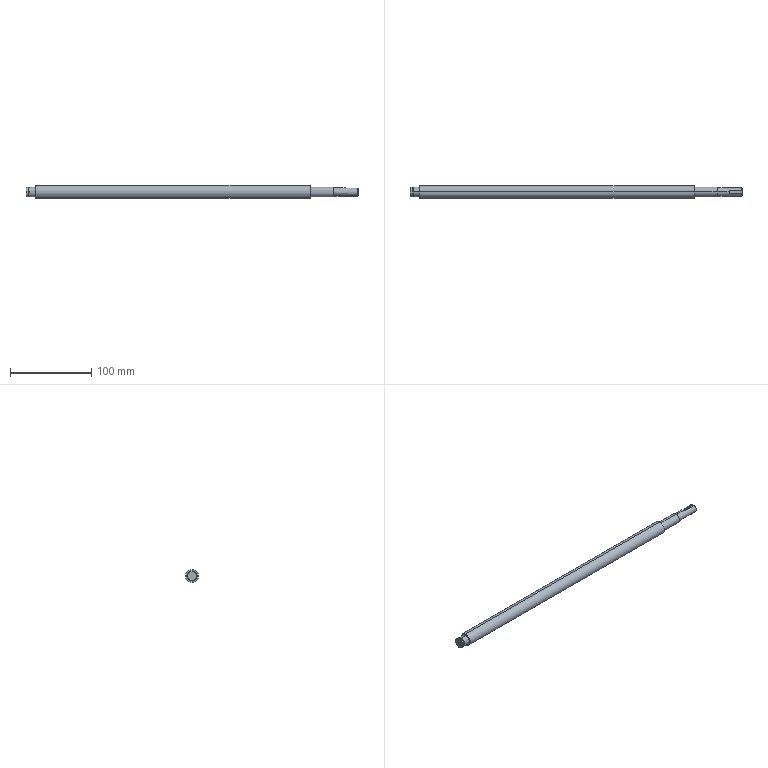Part | SolidWorks | features BaseBody 1 | 1 solid | 34 faces | box 409 x 16 x 16 mm | volume 74846 mm3 | cylinder 13 | plane 10 | torus 6 | cone 5 | commonest cylinder face diameters 12 x6 10 x2 11.5 x2 16 x2 3 x1
STEP:
#1=CARTESIAN_POINT('',(379.3,0.,-5.));
#2=VERTEX_POINT('',#1);
#3=CARTESIAN_POINT('',(379.3,0.,5.));
#4=VERTEX_POINT('',#3);
#5=CARTESIAN_POINT('',(379.3,0.,0.));
#6=DIRECTION('',(1.,0.,0.));
#7=DIRECTION('',(0.,0.,-1.));
#8=AXIS2_PLACEMENT_3D('',#5,#6,#7);
#9=CIRCLE('',#8,5.);
#10=EDGE_CURVE('',#2,#4,#9,.T.);
#11=ORIENTED_EDGE('',*,*,#10,.T.);
#12=CARTESIAN_POINT('',(393.,0.000000043,5.));
#13=VERTEX_POINT('',#12);
#14=CARTESIAN_POINT('',(409.,0.,5.));
#15=DIRECTION('',(1.,0.,0.));
#16=VECTOR('',#15,1000.);
#17=LINE('',#14,#16);
#18=EDGE_CURVE('',#4,#13,#17,.T.);
#19=ORIENTED_EDGE('',*,*,#18,.T.);
#20=CARTESIAN_POINT('',(394.5,1.5,4.77));
#21=VERTEX_POINT('',#20);
#22=CARTESIAN_POINT('',(393.,0.000000043,5.));
#23=CARTESIAN_POINT('',(393.,0.09842,5.));
#24=CARTESIAN_POINT('',(393.01,0.1983,4.997));
#25=CARTESIAN_POINT('',(393.048,0.391,4.986));
#26=CARTESIAN_POINT('',(393.077,0.4848,4.977));
#27=CARTESIAN_POINT('',(393.191,0.758,4.946));
#28=CARTESIAN_POINT('',(393.301,0.9224,4.916));
#29=CARTESIAN_POINT('',(393.509,1.13,4.871));
#30=CARTESIAN_POINT('',(393.584,1.192,4.856));
#31=CARTESIAN_POINT('',(393.746,1.3,4.828));
#32=CARTESIAN_POINT('',(393.833,1.347,4.815));
#33=CARTESIAN_POINT('',(394.104,1.46,4.783));
#34=CARTESIAN_POINT('',(394.301,1.5,4.77));
#35=CARTESIAN_POINT('',(394.5,1.5,4.77));
#36=B_SPLINE_CURVE_WITH_KNOTS('',3,(#22,#23,#24,#25,#26,#27,#28,#29,#30,#31,#32,#33,#34,#35),.UNSPECIFIED.,.F.,.F.,(4,2,2,2,2,2,4),(2.359,2.654,2.948,3.537,3.832,4.126,4.715),.UNSPECIFIED.);
#37=EDGE_CURVE('',#13,#21,#36,.T.);
#38=ORIENTED_EDGE('',*,*,#37,.T.);
#39=CARTESIAN_POINT('',(408.5,1.5,4.77));
#40=VERTEX_POINT('',#39);
#41=CARTESIAN_POINT('',(394.5,1.5,4.77));
#42=DIRECTION('',(1.,0.,0.));
#43=VECTOR('',#42,1000.);
#44=LINE('',#41,#43);
#45=EDGE_CURVE('',#21,#40,#44,.T.);
#46=ORIENTED_EDGE('',*,*,#45,.T.);
#47=CARTESIAN_POINT('',(408.5,0.,-5.));
#48=VERTEX_POINT('',#47);
#49=CARTESIAN_POINT('',(408.5,0.,0.));
#50=DIRECTION('',(1.,0.,0.));
#51=DIRECTION('',(0.,-0.3,0.9539));
#52=AXIS2_PLACEMENT_3D('',#49,#50,#51);
#53=CIRCLE('',#52,5.);
#54=EDGE_CURVE('',#48,#40,#53,.T.);
#55=ORIENTED_EDGE('',*,*,#54,.F.);
#56=CARTESIAN_POINT('',(409.,0.,-5.));
#57=DIRECTION('',(1.,0.,0.));
#58=VECTOR('',#57,1000.);
#59=LINE('',#56,#58);
#60=EDGE_CURVE('',#2,#48,#59,.T.);
#61=ORIENTED_EDGE('',*,*,#60,.F.);
#62=EDGE_LOOP('',(#11,#19,#38,#46,#55,#61));
#63=FACE_OUTER_BOUND('',#62,.T.);
#64=CARTESIAN_POINT('',(409.,0.,0.));
#65=DIRECTION('',(1.,0.,0.));
#66=DIRECTION('',(0.,0.,-1.));
#67=AXIS2_PLACEMENT_3D('',#64,#65,#66);
#68=CYLINDRICAL_SURFACE('',#67,5.);
#69=ADVANCED_FACE('',(#63),#68,.T.);
#70=CARTESIAN_POINT('',(0.,0.,-5.5));
#71=VERTEX_POINT('',#70);
#72=CARTESIAN_POINT('',(0.,0.,5.5));
#73=VERTEX_POINT('',#72);
#74=CARTESIAN_POINT('',(0.,0.,0.));
#75=DIRECTION('',(1.,0.,0.));
#76=DIRECTION('',(0.,0.,-1.));
#77=AXIS2_PLACEMENT_3D('',#74,#75,#76);
#78=CIRCLE('',#77,5.5);
#79=EDGE_CURVE('',#71,#73,#78,.T.);
#80=ORIENTED_EDGE('',*,*,#79,.T.);
#81=CARTESIAN_POINT('',(0.5,0.,6.));
#82=VERTEX_POINT('',#81);
#83=CARTESIAN_POINT('',(0.,0.,5.5));
#84=DIRECTION('',(0.7071,0.,0.7071));
#85=VECTOR('',#84,1000.);
#86=LINE('',#83,#85);
#87=EDGE_CURVE('',#73,#82,#86,.T.);
#88=ORIENTED_EDGE('',*,*,#87,.T.);
#89=CARTESIAN_POINT('',(0.5,0.,-6.));
#90=VERTEX_POINT('',#89);
#91=CARTESIAN_POINT('',(0.5,0.,0.));
#92=DIRECTION('',(1.,0.,0.));
#93=DIRECTION('',(0.,0.,-1.));
#94=AXIS2_PLACEMENT_3D('',#91,#92,#93);
#95=CIRCLE('',#94,6.);
#96=EDGE_CURVE('',#90,#82,#95,.T.);
#97=ORIENTED_EDGE('',*,*,#96,.F.);
#98=CARTESIAN_POINT('',(0.,0.,-5.5));
#99=DIRECTION('',(0.7071,0.,-0.7071));
#100=VECTOR('',#99,1000.);
#101=LINE('',#98,#100);
#102=EDGE_CURVE('',#71,#90,#101,.T.);
#103=ORIENTED_EDGE('',*,*,#102,.F.);
#104=EDGE_LOOP('',(#80,#88,#97,#103));
#105=FACE_OUTER_BOUND('',#104,.T.);
#106=CARTESIAN_POINT('',(0.,0.,0.));
#107=DIRECTION('',(1.,0.,0.));
#108=DIRECTION('',(0.,0.,-1.));
#109=AXIS2_PLACEMENT_3D('',#106,#107,#108);
#110=CONICAL_SURFACE('',#109,5.5,0.7854);
#111=ADVANCED_FACE('',(#105),#110,.T.);
#112=CARTESIAN_POINT('',(379.3,0.,0.));
#113=DIRECTION('',(1.,0.,0.));
#114=DIRECTION('',(0.,0.,-1.));
#115=AXIS2_PLACEMENT_3D('',#112,#113,#114);
#116=CIRCLE('',#115,5.);
#117=EDGE_CURVE('',#4,#2,#116,.T.);
#118=ORIENTED_EDGE('',*,*,#117,.F.);
#119=CARTESIAN_POINT('',(379.,0.,5.3));
#120=VERTEX_POINT('',#119);
#121=CARTESIAN_POINT('',(379.3,0.,5.3));
#122=DIRECTION('',(0.,1.,0.));
#123=DIRECTION('',(0.,0.,1.));
#124=AXIS2_PLACEMENT_3D('',#121,#122,#123);
#125=CIRCLE('',#124,0.3);
#126=EDGE_CURVE('',#4,#120,#125,.T.);
#127=ORIENTED_EDGE('',*,*,#126,.T.);
#128=CARTESIAN_POINT('',(379.,0.,-5.3));
#129=VERTEX_POINT('',#128);
#130=CARTESIAN_POINT('',(379.,0.,0.));
#131=DIRECTION('',(1.,0.,0.));
#132=DIRECTION('',(0.,0.,-1.));
#133=AXIS2_PLACEMENT_3D('',#130,#131,#132);
#134=CIRCLE('',#133,5.3);
#135=EDGE_CURVE('',#120,#129,#134,.T.);
#136=ORIENTED_EDGE('',*,*,#135,.T.);
#137=CARTESIAN_POINT('',(379.3,0.,-5.3));
#138=DIRECTION('',(0.,-1.,0.));
#139=DIRECTION('',(0.,0.,-1.));
#140=AXIS2_PLACEMENT_3D('',#137,#138,#139);
#141=CIRCLE('',#140,0.3);
#142=EDGE_CURVE('',#2,#129,#141,.T.);
#143=ORIENTED_EDGE('',*,*,#142,.F.);
#144=EDGE_LOOP('',(#118,#127,#136,#143));
#145=FACE_OUTER_BOUND('',#144,.T.);
#146=CARTESIAN_POINT('',(379.3,0.,0.));
#147=DIRECTION('',(1.,0.,0.));
#148=DIRECTION('',(0.,0.,-1.));
#149=AXIS2_PLACEMENT_3D('',#146,#147,#148);
#150=TOROIDAL_SURFACE('',#149,5.3,0.3);
#151=ADVANCED_FACE('',(#145),#150,.F.);
#152=ORIENTED_EDGE('',*,*,#96,.T.);
#153=CARTESIAN_POINT('',(2.71,0.,6.));
#154=VERTEX_POINT('',#153);
#155=CARTESIAN_POINT('',(12.,0.,6.));
#156=DIRECTION('',(1.,0.,0.));
#157=VECTOR('',#156,1000.);
#158=LINE('',#155,#157);
#159=EDGE_CURVE('',#82,#154,#158,.T.);
#160=ORIENTED_EDGE('',*,*,#159,.T.);
#161=CARTESIAN_POINT('',(2.71,0.,-6.));
#162=VERTEX_POINT('',#161);
#163=CARTESIAN_POINT('',(2.71,0.,0.));
#164=DIRECTION('',(-1.,0.,0.));
#165=DIRECTION('',(0.,0.,1.));
#166=AXIS2_PLACEMENT_3D('',#163,#164,#165);
#167=CIRCLE('',#166,6.);
#168=EDGE_CURVE('',#154,#162,#167,.T.);
#169=ORIENTED_EDGE('',*,*,#168,.T.);
#170=CARTESIAN_POINT('',(12.,0.,-6.));
#171=DIRECTION('',(1.,0.,0.));
#172=VECTOR('',#171,1000.);
#173=LINE('',#170,#172);
#174=EDGE_CURVE('',#90,#162,#173,.T.);
#175=ORIENTED_EDGE('',*,*,#174,.F.);
#176=EDGE_LOOP('',(#152,#160,#169,#175));
#177=FACE_OUTER_BOUND('',#176,.T.);
#178=CARTESIAN_POINT('',(12.,0.,0.));
#179=DIRECTION('',(1.,0.,0.));
#180=DIRECTION('',(0.,0.,-1.));
#181=AXIS2_PLACEMENT_3D('',#178,#179,#180);
#182=CYLINDRICAL_SURFACE('',#181,6.);
#183=ADVANCED_FACE('',(#177),#182,.T.);
#184=CARTESIAN_POINT('',(379.,0.,-5.387));
#185=VERTEX_POINT('',#184);
#186=CARTESIAN_POINT('',(379.,0.,5.387));
#187=VERTEX_POINT('',#186);
#188=CARTESIAN_POINT('',(379.,0.,0.));
#189=DIRECTION('',(1.,0.,0.));
#190=DIRECTION('',(0.,0.,-1.));
#191=AXIS2_PLACEMENT_3D('',#188,#189,#190);
#192=CIRCLE('',#191,5.387);
#193=EDGE_CURVE('',#185,#187,#192,.T.);
#194=ORIENTED_EDGE('',*,*,#193,.F.);
#195=CARTESIAN_POINT('',(378.387,0.,-6.));
#196=VERTEX_POINT('',#195);
#197=CARTESIAN_POINT('',(378.387,0.,-6.));
#198=DIRECTION('',(-0.7071,0.,-0.7071));
#199=VECTOR('',#198,1000.);
#200=LINE('',#197,#199);
#201=EDGE_CURVE('',#185,#196,#200,.T.);
#202=ORIENTED_EDGE('',*,*,#201,.T.);
#203=CARTESIAN_POINT('',(378.387,0.,6.));
#204=VERTEX_POINT('',#203);
#205=CARTESIAN_POINT('',(378.387,0.,0.));
#206=DIRECTION('',(1.,0.,0.));
#207=DIRECTION('',(0.,0.,-1.));
#208=AXIS2_PLACEMENT_3D('',#205,#206,#207);
#209=CIRCLE('',#208,6.);
#210=EDGE_CURVE('',#196,#204,#209,.T.);
#211=ORIENTED_EDGE('',*,*,#210,.T.);
#212=CARTESIAN_POINT('',(378.387,0.,6.));
#213=DIRECTION('',(-0.7071,0.,0.7071));
#214=VECTOR('',#213,1000.);
#215=LINE('',#212,#214);
#216=EDGE_CURVE('',#187,#204,#215,.T.);
#217=ORIENTED_EDGE('',*,*,#216,.F.);
#218=EDGE_LOOP('',(#194,#202,#211,#217));
#219=FACE_OUTER_BOUND('',#218,.T.);
#220=CARTESIAN_POINT('',(378.387,0.,0.));
#221=DIRECTION('',(-1.,0.,0.));
#222=DIRECTION('',(0.,0.,1.));
#223=AXIS2_PLACEMENT_3D('',#220,#221,#222);
#224=CONICAL_SURFACE('',#223,6.,0.7854);
#225=ADVANCED_FACE('',(#219),#224,.T.);
#226=CARTESIAN_POINT('',(2.71,0.,-5.75));
#227=VERTEX_POINT('',#226);
#228=CARTESIAN_POINT('',(2.71,0.,5.75));
#229=VERTEX_POINT('',#228);
#230=CARTESIAN_POINT('',(2.71,0.,0.));
#231=DIRECTION('',(1.,0.,0.));
#232=DIRECTION('',(0.,0.,-1.));
#233=AXIS2_PLACEMENT_3D('',#230,#231,#232);
#234=CIRCLE('',#233,5.75);
#235=EDGE_CURVE('',#227,#229,#234,.T.);
#236=ORIENTED_EDGE('',*,*,#235,.T.);
#237=CARTESIAN_POINT('',(4.,0.,5.75));
#238=VERTEX_POINT('',#237);
#239=CARTESIAN_POINT('',(409.,0.,5.75));
#240=DIRECTION('',(1.,0.,0.));
#241=VECTOR('',#240,1000.);
#242=LINE('',#239,#241);
#243=EDGE_CURVE('',#229,#238,#242,.T.);
#244=ORIENTED_EDGE('',*,*,#243,.T.);
#245=CARTESIAN_POINT('',(4.,0.,-5.75));
#246=VERTEX_POINT('',#245);
#247=CARTESIAN_POINT('',(4.,0.,0.));
#248=DIRECTION('',(1.,0.,0.));
#249=DIRECTION('',(0.,0.,-1.));
#250=AXIS2_PLACEMENT_3D('',#247,#248,#249);
#251=CIRCLE('',#250,5.75);
#252=EDGE_CURVE('',#246,#238,#251,.T.);
#253=ORIENTED_EDGE('',*,*,#252,.F.);
#254=CARTESIAN_POINT('',(409.,0.,-5.75));
#255=DIRECTION('',(1.,0.,0.));
#256=VECTOR('',#255,1000.);
#257=LINE('',#254,#256);
#258=EDGE_CURVE('',#227,#246,#257,.T.);
#259=ORIENTED_EDGE('',*,*,#258,.F.);
#260=EDGE_LOOP('',(#236,#244,#253,#259));
#261=FACE_OUTER_BOUND('',#260,.T.);
#262=CARTESIAN_POINT('',(409.,0.,0.));
#263=DIRECTION('',(1.,0.,0.));
#264=DIRECTION('',(0.,0.,-1.));
#265=AXIS2_PLACEMENT_3D('',#262,#263,#264);
#266=CYLINDRICAL_SURFACE('',#265,5.75);
#267=ADVANCED_FACE('',(#261),#266,.T.);
#268=CARTESIAN_POINT('',(350.3,0.,-6.));
#269=VERTEX_POINT('',#268);
#270=CARTESIAN_POINT('',(350.3,0.,6.));
#271=VERTEX_POINT('',#270);
#272=CARTESIAN_POINT('',(350.3,0.,0.));
#273=DIRECTION('',(1.,0.,0.));
#274=DIRECTION('',(0.,0.,-1.));
#275=AXIS2_PLACEMENT_3D('',#272,#273,#274);
#276=CIRCLE('',#275,6.);
#277=EDGE_CURVE('',#269,#271,#276,.T.);
#278=ORIENTED_EDGE('',*,*,#277,.T.);
#279=CARTESIAN_POINT('',(409.,0.,6.));
#280=DIRECTION('',(1.,0.,0.));
#281=VECTOR('',#280,1000.);
#282=LINE('',#279,#281);
#283=EDGE_CURVE('',#271,#204,#282,.T.);
#284=ORIENTED_EDGE('',*,*,#283,.T.);
#285=ORIENTED_EDGE('',*,*,#210,.F.);
#286=CARTESIAN_POINT('',(409.,0.,-6.));
#287=DIRECTION('',(1.,0.,0.));
#288=VECTOR('',#287,1000.);
#289=LINE('',#286,#288);
#290=EDGE_CURVE('',#269,#196,#289,.T.);
#291=ORIENTED_EDGE('',*,*,#290,.F.);
#292=EDGE_LOOP('',(#278,#284,#285,#291));
#293=FACE_OUTER_BOUND('',#292,.T.);
#294=CARTESIAN_POINT('',(409.,0.,0.));
#295=DIRECTION('',(1.,0.,0.));
#296=DIRECTION('',(0.,0.,-1.));
#297=AXIS2_PLACEMENT_3D('',#294,#295,#296);
#298=CYLINDRICAL_SURFACE('',#297,6.);
#299=ADVANCED_FACE('',(#293),#298,.T.);
#300=CARTESIAN_POINT('',(350.3,0.,0.));
#301=DIRECTION('',(1.,0.,0.));
#302=DIRECTION('',(0.,0.,-1.));
#303=AXIS2_PLACEMENT_3D('',#300,#301,#302);
#304=CIRCLE('',#303,6.);
#305=EDGE_CURVE('',#271,#269,#304,.T.);
#306=ORIENTED_EDGE('',*,*,#305,.F.);
#307=CARTESIAN_POINT('',(350.,0.,6.3));
#308=VERTEX_POINT('',#307);
#309=CARTESIAN_POINT('',(350.3,0.,6.3));
#310=DIRECTION('',(0.,1.,0.));
#311=DIRECTION('',(0.,0.,1.));
#312=AXIS2_PLACEMENT_3D('',#309,#310,#311);
#313=CIRCLE('',#312,0.3);
#314=EDGE_CURVE('',#271,#308,#313,.T.);
#315=ORIENTED_EDGE('',*,*,#314,.T.);
#316=CARTESIAN_POINT('',(350.,0.,-6.3));
#317=VERTEX_POINT('',#316);
#318=CARTESIAN_POINT('',(350.,0.,0.));
#319=DIRECTION('',(1.,0.,0.));
#320=DIRECTION('',(0.,0.,-1.));
#321=AXIS2_PLACEMENT_3D('',#318,#319,#320);
#322=CIRCLE('',#321,6.3);
#323=EDGE_CURVE('',#308,#317,#322,.T.);
#324=ORIENTED_EDGE('',*,*,#323,.T.);
#325=CARTESIAN_POINT('',(350.3,0.,-6.3));
#326=DIRECTION('',(0.,-1.,0.));
#327=DIRECTION('',(0.,0.,-1.));
#328=AXIS2_PLACEMENT_3D('',#325,#326,#327);
#329=CIRCLE('',#328,0.3);
#330=EDGE_CURVE('',#269,#317,#329,.T.);
#331=ORIENTED_EDGE('',*,*,#330,.F.);
#332=EDGE_LOOP('',(#306,#315,#324,#331));
#333=FACE_OUTER_BOUND('',#332,.T.);
#334=CARTESIAN_POINT('',(350.3,0.,0.));
#335=DIRECTION('',(1.,0.,0.));
#336=DIRECTION('',(0.,0.,-1.));
#337=AXIS2_PLACEMENT_3D('',#334,#335,#336);
#338=TOROIDAL_SURFACE('',#337,6.3,0.3);
#339=ADVANCED_FACE('',(#333),#338,.F.);
#340=CARTESIAN_POINT('',(4.,0.,-6.));
#341=VERTEX_POINT('',#340);
#342=CARTESIAN_POINT('',(4.,0.,6.));
#343=VERTEX_POINT('',#342);
#344=CARTESIAN_POINT('',(4.,0.,0.));
#345=DIRECTION('',(1.,0.,0.));
#346=DIRECTION('',(0.,0.,-1.));
#347=AXIS2_PLACEMENT_3D('',#344,#345,#346);
#348=CIRCLE('',#347,6.);
#349=EDGE_CURVE('',#341,#343,#348,.T.);
#350=ORIENTED_EDGE('',*,*,#349,.T.);
#351=CARTESIAN_POINT('',(11.7,0.,6.));
#352=VERTEX_POINT('',#351);
#353=CARTESIAN_POINT('',(12.,0.,6.));
#354=DIRECTION('',(1.,0.,0.));
#355=VECTOR('',#354,1000.);
#356=LINE('',#353,#355);
#357=EDGE_CURVE('',#343,#352,#356,.T.);
#358=ORIENTED_EDGE('',*,*,#357,.T.);
#359=CARTESIAN_POINT('',(11.7,0.,-6.));
#360=VERTEX_POINT('',#359);
#361=CARTESIAN_POINT('',(11.7,0.,0.));
#362=DIRECTION('',(1.,0.,0.));
#363=DIRECTION('',(0.,0.,-1.));
#364=AXIS2_PLACEMENT_3D('',#361,#362,#363);
#365=CIRCLE('',#364,6.);
#366=EDGE_CURVE('',#360,#352,#365,.T.);
#367=ORIENTED_EDGE('',*,*,#366,.F.);
#368=CARTESIAN_POINT('',(12.,0.,-6.));
#369=DIRECTION('',(1.,0.,0.));
#370=VECTOR('',#369,1000.);
#371=LINE('',#368,#370);
#372=EDGE_CURVE('',#341,#360,#371,.T.);
#373=ORIENTED_EDGE('',*,*,#372,.F.);
#374=EDGE_LOOP('',(#350,#358,#367,#373));
#375=FACE_OUTER_BOUND('',#374,.T.);
#376=CARTESIAN_POINT('',(12.,0.,0.));
#377=DIRECTION('',(1.,0.,0.));
#378=DIRECTION('',(0.,0.,-1.));
#379=AXIS2_PLACEMENT_3D('',#376,#377,#378);
#380=CYLINDRICAL_SURFACE('',#379,6.);
#381=ADVANCED_FACE('',(#375),#380,.T.);
#382=CARTESIAN_POINT('',(12.,0.,6.3));
#383=VERTEX_POINT('',#382);
#384=CARTESIAN_POINT('',(12.,0.,-6.3));
#385=VERTEX_POINT('',#384);
#386=CARTESIAN_POINT('',(12.,0.,0.));
#387=DIRECTION('',(1.,0.,0.));
#388=DIRECTION('',(0.,0.,-1.));
#389=AXIS2_PLACEMENT_3D('',#386,#387,#388);
#390=CIRCLE('',#389,6.3);
#391=EDGE_CURVE('',#383,#385,#390,.T.);
#392=ORIENTED_EDGE('',*,*,#391,.F.);
#393=CARTESIAN_POINT('',(11.7,0.,6.3));
#394=DIRECTION('',(0.,1.,0.));
#395=DIRECTION('',(0.,0.,1.));
#396=AXIS2_PLACEMENT_3D('',#393,#394,#395);
#397=CIRCLE('',#396,0.3);
#398=EDGE_CURVE('',#383,#352,#397,.T.);
#399=ORIENTED_EDGE('',*,*,#398,.T.);
#400=CARTESIAN_POINT('',(11.7,0.,0.));
#401=DIRECTION('',(1.,0.,0.));
#402=DIRECTION('',(0.,0.,-1.));
#403=AXIS2_PLACEMENT_3D('',#400,#401,#402);
#404=CIRCLE('',#403,6.);
#405=EDGE_CURVE('',#352,#360,#404,.T.);
#406=ORIENTED_EDGE('',*,*,#405,.T.);
#407=CARTESIAN_POINT('',(11.7,0.,-6.3));
#408=DIRECTION('',(0.,-1.,0.));
#409=DIRECTION('',(0.,0.,-1.));
#410=AXIS2_PLACEMENT_3D('',#407,#408,#409);
#411=CIRCLE('',#410,0.3);
#412=EDGE_CURVE('',#385,#360,#411,.T.);
#413=ORIENTED_EDGE('',*,*,#412,.F.);
#414=EDGE_LOOP('',(#392,#399,#406,#413));
#415=FACE_OUTER_BOUND('',#414,.T.);
#416=CARTESIAN_POINT('',(11.7,0.,0.));
#417=DIRECTION('',(1.,0.,0.));
#418=DIRECTION('',(0.,0.,-1.));
#419=AXIS2_PLACEMENT_3D('',#416,#417,#418);
#420=TOROIDAL_SURFACE('',#419,6.3,0.3);
#421=ADVANCED_FACE('',(#415),#420,.F.);
#422=CARTESIAN_POINT('',(12.,0.,-8.));
#423=VERTEX_POINT('',#422);
#424=CARTESIAN_POINT('',(12.,0.,8.));
#425=VERTEX_POINT('',#424);
#426=CARTESIAN_POINT('',(12.,0.,0.));
#427=DIRECTION('',(1.,0.,0.));
#428=DIRECTION('',(0.,0.,-1.));
#429=AXIS2_PLACEMENT_3D('',#426,#427,#428);
#430=CIRCLE('',#429,8.);
#431=EDGE_CURVE('',#423,#425,#430,.T.);
#432=ORIENTED_EDGE('',*,*,#431,.T.);
#433=CARTESIAN_POINT('',(350.,0.,8.));
#434=VERTEX_POINT('',#433);
#435=CARTESIAN_POINT('',(350.,0.,8.));
#436=DIRECTION('',(1.,0.,0.));
#437=VECTOR('',#436,1000.);
#438=LINE('',#435,#437);
#439=EDGE_CURVE('',#425,#434,#438,.T.);
#440=ORIENTED_EDGE('',*,*,#439,.T.);
#441=CARTESIAN_POINT('',(350.,0.,-8.));
#442=VERTEX_POINT('',#441);
#443=CARTESIAN_POINT('',(350.,0.,0.));
#444=DIRECTION('',(1.,0.,0.));
#445=DIRECTION('',(0.,0.,-1.));
#446=AXIS2_PLACEMENT_3D('',#443,#444,#445);
#447=CIRCLE('',#446,8.);
#448=EDGE_CURVE('',#442,#434,#447,.T.);
#449=ORIENTED_EDGE('',*,*,#448,.F.);
#450=CARTESIAN_POINT('',(350.,0.,-8.));
#451=DIRECTION('',(1.,0.,0.));
#452=VECTOR('',#451,1000.);
#453=LINE('',#450,#452);
#454=EDGE_CURVE('',#423,#442,#453,.T.);
#455=ORIENTED_EDGE('',*,*,#454,.F.);
#456=EDGE_LOOP('',(#432,#440,#449,#455));
#457=FACE_OUTER_BOUND('',#456,.T.);
#458=CARTESIAN_POINT('',(350.,0.,0.));
#459=DIRECTION('',(1.,0.,0.));
#460=DIRECTION('',(0.,0.,-1.));
#461=AXIS2_PLACEMENT_3D('',#458,#459,#460);
#462=CYLINDRICAL_SURFACE('',#461,8.);
#463=ADVANCED_FACE('',(#457),#462,.T.);
#464=ORIENTED_EDGE('',*,*,#431,.F.);
#465=CARTESIAN_POINT('',(12.,0.,0.));
#466=DIRECTION('',(1.,0.,0.));
#467=DIRECTION('',(0.,0.,-1.));
#468=AXIS2_PLACEMENT_3D('',#465,#466,#467);
#469=CIRCLE('',#468,8.);
#470=EDGE_CURVE('',#425,#423,#469,.T.);
#471=ORIENTED_EDGE('',*,*,#470,.F.);
#472=EDGE_LOOP('',(#464,#471));
#473=FACE_OUTER_BOUND('',#472,.T.);
#474=CARTESIAN_POINT('',(12.,0.,0.));
#475=DIRECTION('',(1.,0.,0.));
#476=DIRECTION('',(0.,0.,-1.));
#477=AXIS2_PLACEMENT_3D('',#474,#475,#476);
#478=CIRCLE('',#477,6.3);
#479=EDGE_CURVE('',#385,#383,#478,.T.);
#480=ORIENTED_EDGE('',*,*,#479,.T.);
#481=ORIENTED_EDGE('',*,*,#391,.T.);
#482=EDGE_LOOP('',(#480,#481));
#483=FACE_BOUND('',#482,.T.);
#484=CARTESIAN_POINT('',(12.,0.,0.));
#485=DIRECTION('',(1.,0.,0.));
#486=DIRECTION('',(0.,0.,-1.));
#487=AXIS2_PLACEMENT_3D('',#484,#485,#486);
#488=PLANE('',#487);
#489=ADVANCED_FACE('',(#473,#483),#488,.F.);
#490=ORIENTED_EDGE('',*,*,#439,.F.);
#491=ORIENTED_EDGE('',*,*,#470,.T.);
#492=ORIENTED_EDGE('',*,*,#454,.T.);
#493=CARTESIAN_POINT('',(350.,0.,0.));
#494=DIRECTION('',(1.,0.,0.));
#495=DIRECTION('',(0.,0.,-1.));
#496=AXIS2_PLACEMENT_3D('',#493,#494,#495);
#497=CIRCLE('',#496,8.);
#498=EDGE_CURVE('',#434,#442,#497,.T.);
#499=ORIENTED_EDGE('',*,*,#498,.F.);
#500=EDGE_LOOP('',(#490,#491,#492,#499));
#501=FACE_OUTER_BOUND('',#500,.T.);
#502=CARTESIAN_POINT('',(350.,0.,0.));
#503=DIRECTION('',(1.,0.,0.));
#504=DIRECTION('',(0.,0.,-1.));
#505=AXIS2_PLACEMENT_3D('',#502,#503,#504);
#506=CYLINDRICAL_SURFACE('',#505,8.);
#507=ADVANCED_FACE('',(#501),#506,.T.);
#508=ORIENTED_EDGE('',*,*,#398,.F.);
#509=ORIENTED_EDGE('',*,*,#479,.F.);
#510=ORIENTED_EDGE('',*,*,#412,.T.);
#511=ORIENTED_EDGE('',*,*,#366,.T.);
#512=EDGE_LOOP('',(#508,#509,#510,#511));
#513=FACE_OUTER_BOUND('',#512,.T.);
#514=CARTESIAN_POINT('',(11.7,0.,0.));
#515=DIRECTION('',(1.,0.,0.));
#516=DIRECTION('',(0.,0.,-1.));
#517=AXIS2_PLACEMENT_3D('',#514,#515,#516);
#518=TOROIDAL_SURFACE('',#517,6.3,0.3);
#519=ADVANCED_FACE('',(#513),#518,.F.);
#520=CARTESIAN_POINT('',(350.,0.,0.));
#521=DIRECTION('',(1.,0.,0.));
#522=DIRECTION('',(0.,0.,-1.));
#523=AXIS2_PLACEMENT_3D('',#520,#521,#522);
#524=CIRCLE('',#523,6.3);
#525=EDGE_CURVE('',#317,#308,#524,.T.);
#526=ORIENTED_EDGE('',*,*,#525,.F.);
#527=ORIENTED_EDGE('',*,*,#323,.F.);
#528=EDGE_LOOP('',(#526,#527));
#529=FACE_BOUND('',#528,.T.);
#530=ORIENTED_EDGE('',*,*,#448,.T.);
#531=ORIENTED_EDGE('',*,*,#498,.T.);
#532=EDGE_LOOP('',(#530,#531));
#533=FACE_OUTER_BOUND('',#532,.T.);
#534=CARTESIAN_POINT('',(350.,8.,0.));
#535=DIRECTION('',(-1.,0.,0.));
#536=DIRECTION('',(0.,0.,1.));
#537=AXIS2_PLACEMENT_3D('',#534,#535,#536);
#538=PLANE('',#537);
#539=ADVANCED_FACE('',(#529,#533),#538,.F.);
#540=ORIENTED_EDGE('',*,*,#357,.F.);
#541=CARTESIAN_POINT('',(4.,0.,0.));
#542=DIRECTION('',(1.,0.,0.));
#543=DIRECTION('',(0.,0.,-1.));
#544=AXIS2_PLACEMENT_3D('',#541,#542,#543);
#545=CIRCLE('',#544,6.);
#546=EDGE_CURVE('',#343,#341,#545,.T.);
#547=ORIENTED_EDGE('',*,*,#546,.T.);
#548=ORIENTED_EDGE('',*,*,#372,.T.);
#549=ORIENTED_EDGE('',*,*,#405,.F.);
#550=EDGE_LOOP('',(#540,#547,#548,#549));
#551=FACE_OUTER_BOUND('',#550,.T.);
#552=CARTESIAN_POINT('',(12.,0.,0.));
#553=DIRECTION('',(1.,0.,0.));
#554=DIRECTION('',(0.,0.,-1.));
#555=AXIS2_PLACEMENT_3D('',#552,#553,#554);
#556=CYLINDRICAL_SURFACE('',#555,6.);
#557=ADVANCED_FACE('',(#551),#556,.T.);
#558=ORIENTED_EDGE('',*,*,#314,.F.);
#559=ORIENTED_EDGE('',*,*,#277,.F.);
#560=ORIENTED_EDGE('',*,*,#330,.T.);
#561=ORIENTED_EDGE('',*,*,#525,.T.);
#562=EDGE_LOOP('',(#558,#559,#560,#561));
#563=FACE_OUTER_BOUND('',#562,.T.);
#564=CARTESIAN_POINT('',(350.3,0.,0.));
#565=DIRECTION('',(1.,0.,0.));
#566=DIRECTION('',(0.,0.,-1.));
#567=AXIS2_PLACEMENT_3D('',#564,#565,#566);
#568=TOROIDAL_SURFACE('',#567,6.3,0.3);
#569=ADVANCED_FACE('',(#563),#568,.F.);
#570=ORIENTED_EDGE('',*,*,#349,.F.);
#571=ORIENTED_EDGE('',*,*,#546,.F.);
#572=EDGE_LOOP('',(#570,#571));
#573=FACE_OUTER_BOUND('',#572,.T.);
#574=ORIENTED_EDGE('',*,*,#252,.T.);
#575=CARTESIAN_POINT('',(4.,0.,0.));
#576=DIRECTION('',(1.,0.,0.));
#577=DIRECTION('',(0.,0.,-1.));
#578=AXIS2_PLACEMENT_3D('',#575,#576,#577);
#579=CIRCLE('',#578,5.75);
#580=EDGE_CURVE('',#238,#246,#579,.T.);
#581=ORIENTED_EDGE('',*,*,#580,.T.);
#582=EDGE_LOOP('',(#574,#581));
#583=FACE_BOUND('',#582,.T.);
#584=CARTESIAN_POINT('',(4.,5.75,0.));
#585=DIRECTION('',(1.,0.,0.));
#586=DIRECTION('',(0.,0.,-1.));
#587=AXIS2_PLACEMENT_3D('',#584,#585,#586);
#588=PLANE('',#587);
#589=ADVANCED_FACE('',(#573,#583),#588,.F.);
#590=ORIENTED_EDGE('',*,*,#283,.F.);
#591=ORIENTED_EDGE('',*,*,#305,.T.);
#592=ORIENTED_EDGE('',*,*,#290,.T.);
#593=CARTESIAN_POINT('',(378.387,0.,0.));
#594=DIRECTION('',(1.,0.,0.));
#595=DIRECTION('',(0.,0.,-1.));
#596=AXIS2_PLACEMENT_3D('',#593,#594,#595);
#597=CIRCLE('',#596,6.);
#598=EDGE_CURVE('',#204,#196,#597,.T.);
#599=ORIENTED_EDGE('',*,*,#598,.F.);
#600=EDGE_LOOP('',(#590,#591,#592,#599));
#601=FACE_OUTER_BOUND('',#600,.T.);
#602=CARTESIAN_POINT('',(409.,0.,0.));
#603=DIRECTION('',(1.,0.,0.));
#604=DIRECTION('',(0.,0.,-1.));
#605=AXIS2_PLACEMENT_3D('',#602,#603,#604);
#606=CYLINDRICAL_SURFACE('',#605,6.);
#607=ADVANCED_FACE('',(#601),#606,.T.);
#608=ORIENTED_EDGE('',*,*,#243,.F.);
#609=CARTESIAN_POINT('',(2.71,0.,0.));
#610=DIRECTION('',(1.,0.,0.));
#611=DIRECTION('',(0.,0.,-1.));
#612=AXIS2_PLACEMENT_3D('',#609,#610,#611);
#613=CIRCLE('',#612,5.75);
#614=EDGE_CURVE('',#229,#227,#613,.T.);
#615=ORIENTED_EDGE('',*,*,#614,.T.);
#616=ORIENTED_EDGE('',*,*,#258,.T.);
#617=ORIENTED_EDGE('',*,*,#580,.F.);
#618=EDGE_LOOP('',(#608,#615,#616,#617));
#619=FACE_OUTER_BOUND('',#618,.T.);
#620=CARTESIAN_POINT('',(409.,0.,0.));
#621=DIRECTION('',(1.,0.,0.));
#622=DIRECTION('',(0.,0.,-1.));
#623=AXIS2_PLACEMENT_3D('',#620,#621,#622);
#624=CYLINDRICAL_SURFACE('',#623,5.75);
#625=ADVANCED_FACE('',(#619),#624,.T.);
#626=ORIENTED_EDGE('',*,*,#201,.F.);
#627=CARTESIAN_POINT('',(379.,0.,0.));
#628=DIRECTION('',(1.,0.,0.));
#629=DIRECTION('',(0.,0.,-1.));
#630=AXIS2_PLACEMENT_3D('',#627,#628,#629);
#631=CIRCLE('',#630,5.387);
#632=EDGE_CURVE('',#187,#185,#631,.T.);
#633=ORIENTED_EDGE('',*,*,#632,.F.);
#634=ORIENTED_EDGE('',*,*,#216,.T.);
#635=ORIENTED_EDGE('',*,*,#598,.T.);
#636=EDGE_LOOP('',(#626,#633,#634,#635));
#637=FACE_OUTER_BOUND('',#636,.T.);
#638=CARTESIAN_POINT('',(378.387,0.,0.));
#639=DIRECTION('',(-1.,0.,0.));
#640=DIRECTION('',(0.,0.,1.));
#641=AXIS2_PLACEMENT_3D('',#638,#639,#640);
#642=CONICAL_SURFACE('',#641,6.,0.7854);
#643=ADVANCED_FACE('',(#637),#642,.T.);
#644=ORIENTED_EDGE('',*,*,#235,.F.);
#645=ORIENTED_EDGE('',*,*,#614,.F.);
#646=EDGE_LOOP('',(#644,#645));
#647=FACE_BOUND('',#646,.T.);
#648=CARTESIAN_POINT('',(2.71,0.,0.));
#649=DIRECTION('',(-1.,0.,0.));
#650=DIRECTION('',(0.,0.,1.));
#651=AXIS2_PLACEMENT_3D('',#648,#649,#650);
#652=CIRCLE('',#651,6.);
#653=EDGE_CURVE('',#162,#154,#652,.T.);
#654=ORIENTED_EDGE('',*,*,#653,.F.);
#655=ORIENTED_EDGE('',*,*,#168,.F.);
#656=EDGE_LOOP('',(#654,#655));
#657=FACE_OUTER_BOUND('',#656,.T.);
#658=CARTESIAN_POINT('',(2.71,21.75,0.));
#659=DIRECTION('',(-1.,0.,0.));
#660=DIRECTION('',(0.,0.,1.));
#661=AXIS2_PLACEMENT_3D('',#658,#659,#660);
#662=PLANE('',#661);
#663=ADVANCED_FACE('',(#647,#657),#662,.F.);
#664=CARTESIAN_POINT('',(379.,0.,0.));
#665=DIRECTION('',(1.,0.,0.));
#666=DIRECTION('',(0.,0.,-1.));
#667=AXIS2_PLACEMENT_3D('',#664,#665,#666);
#668=CIRCLE('',#667,5.3);
#669=EDGE_CURVE('',#129,#120,#668,.T.);
#670=ORIENTED_EDGE('',*,*,#669,.F.);
#671=ORIENTED_EDGE('',*,*,#135,.F.);
#672=EDGE_LOOP('',(#670,#671));
#673=FACE_BOUND('',#672,.T.);
#674=ORIENTED_EDGE('',*,*,#632,.T.);
#675=ORIENTED_EDGE('',*,*,#193,.T.);
#676=EDGE_LOOP('',(#674,#675));
#677=FACE_OUTER_BOUND('',#676,.T.);
#678=CARTESIAN_POINT('',(379.,5.386,0.));
#679=DIRECTION('',(-1.,0.,0.));
#680=DIRECTION('',(0.,0.,1.));
#681=AXIS2_PLACEMENT_3D('',#678,#679,#680);
#682=PLANE('',#681);
#683=ADVANCED_FACE('',(#673,#677),#682,.F.);
#684=ORIENTED_EDGE('',*,*,#159,.F.);
#685=CARTESIAN_POINT('',(0.5,0.,0.));
#686=DIRECTION('',(1.,0.,0.));
#687=DIRECTION('',(0.,0.,-1.));
#688=AXIS2_PLACEMENT_3D('',#685,#686,#687);
#689=CIRCLE('',#688,6.);
#690=EDGE_CURVE('',#82,#90,#689,.T.);
#691=ORIENTED_EDGE('',*,*,#690,.T.);
#692=ORIENTED_EDGE('',*,*,#174,.T.);
#693=ORIENTED_EDGE('',*,*,#653,.T.);
#694=EDGE_LOOP('',(#684,#691,#692,#693));
#695=FACE_OUTER_BOUND('',#694,.T.);
#696=CARTESIAN_POINT('',(12.,0.,0.));
#697=DIRECTION('',(1.,0.,0.));
#698=DIRECTION('',(0.,0.,-1.));
#699=AXIS2_PLACEMENT_3D('',#696,#697,#698);
#700=CYLINDRICAL_SURFACE('',#699,6.);
#701=ADVANCED_FACE('',(#695),#700,.T.);
#702=ORIENTED_EDGE('',*,*,#126,.F.);
#703=ORIENTED_EDGE('',*,*,#10,.F.);
#704=ORIENTED_EDGE('',*,*,#142,.T.);
#705=ORIENTED_EDGE('',*,*,#669,.T.);
#706=EDGE_LOOP('',(#702,#703,#704,#705));
#707=FACE_OUTER_BOUND('',#706,.T.);
#708=CARTESIAN_POINT('',(379.3,0.,0.));
#709=DIRECTION('',(1.,0.,0.));
#710=DIRECTION('',(0.,0.,-1.));
#711=AXIS2_PLACEMENT_3D('',#708,#709,#710);
#712=TOROIDAL_SURFACE('',#711,5.3,0.3);
#713=ADVANCED_FACE('',(#707),#712,.F.);
#714=ORIENTED_EDGE('',*,*,#87,.F.);
#715=CARTESIAN_POINT('',(0.,0.,0.));
#716=DIRECTION('',(1.,0.,0.));
#717=DIRECTION('',(0.,0.,-1.));
#718=AXIS2_PLACEMENT_3D('',#715,#716,#717);
#719=CIRCLE('',#718,5.5);
#720=EDGE_CURVE('',#73,#71,#719,.T.);
#721=ORIENTED_EDGE('',*,*,#720,.T.);
#722=ORIENTED_EDGE('',*,*,#102,.T.);
#723=ORIENTED_EDGE('',*,*,#690,.F.);
#724=EDGE_LOOP('',(#714,#721,#722,#723));
#725=FACE_OUTER_BOUND('',#724,.T.);
#726=CARTESIAN_POINT('',(0.,0.,0.));
#727=DIRECTION('',(1.,0.,0.));
#728=DIRECTION('',(0.,0.,-1.));
#729=AXIS2_PLACEMENT_3D('',#726,#727,#728);
#730=CONICAL_SURFACE('',#729,5.5,0.7854);
#731=ADVANCED_FACE('',(#725),#730,.T.);
#732=ORIENTED_EDGE('',*,*,#18,.F.);
#733=ORIENTED_EDGE('',*,*,#117,.T.);
#734=ORIENTED_EDGE('',*,*,#60,.T.);
#735=CARTESIAN_POINT('',(408.5,-1.5,4.77));
#736=VERTEX_POINT('',#735);
#737=CARTESIAN_POINT('',(408.5,0.,0.));
#738=DIRECTION('',(1.,0.,0.));
#739=DIRECTION('',(0.,-0.3,0.9539));
#740=AXIS2_PLACEMENT_3D('',#737,#738,#739);
#741=CIRCLE('',#740,5.);
#742=EDGE_CURVE('',#736,#48,#741,.T.);
#743=ORIENTED_EDGE('',*,*,#742,.F.);
#744=CARTESIAN_POINT('',(394.5,-1.5,4.77));
#745=VERTEX_POINT('',#744);
#746=CARTESIAN_POINT('',(408.5,-1.5,4.77));
#747=DIRECTION('',(-1.,0.,0.));
#748=VECTOR('',#747,1000.);
#749=LINE('',#746,#748);
#750=EDGE_CURVE('',#736,#745,#749,.T.);
#751=ORIENTED_EDGE('',*,*,#750,.T.);
#752=CARTESIAN_POINT('',(394.5,-1.5,4.77));
#753=CARTESIAN_POINT('',(394.4,-1.5,4.77));
#754=CARTESIAN_POINT('',(394.302,-1.49,4.773));
#755=CARTESIAN_POINT('',(394.11,-1.452,4.785));
#756=CARTESIAN_POINT('',(394.014,-1.423,4.794));
#757=CARTESIAN_POINT('',(393.833,-1.347,4.815));
#758=CARTESIAN_POINT('',(393.747,-1.301,4.828));
#759=CARTESIAN_POINT('',(393.584,-1.192,4.856));
#760=CARTESIAN_POINT('',(393.508,-1.129,4.871));
#761=CARTESIAN_POINT('',(393.301,-0.9228,4.916));
#762=CARTESIAN_POINT('',(393.19,-0.7562,4.946));
#763=CARTESIAN_POINT('',(393.04,-0.3953,4.988));
#764=CARTESIAN_POINT('',(393.,-0.1971,5.));
#765=CARTESIAN_POINT('',(393.,0.000000043,5.));
#766=B_SPLINE_CURVE_WITH_KNOTS('',3,(#752,#753,#754,#755,#756,#757,#758,#759,#760,#761,#762,#763,#764,#765),.UNSPECIFIED.,.F.,.F.,(4,2,2,2,2,2,4),(0.,0.2949,0.5898,0.8847,1.18,1.769,2.359),.UNSPECIFIED.);
#767=EDGE_CURVE('',#745,#13,#766,.T.);
#768=ORIENTED_EDGE('',*,*,#767,.T.);
#769=EDGE_LOOP('',(#732,#733,#734,#743,#751,#768));
#770=FACE_OUTER_BOUND('',#769,.T.);
#771=CARTESIAN_POINT('',(409.,0.,0.));
#772=DIRECTION('',(1.,0.,0.));
#773=DIRECTION('',(0.,0.,-1.));
#774=AXIS2_PLACEMENT_3D('',#771,#772,#773);
#775=CYLINDRICAL_SURFACE('',#774,5.);
#776=ADVANCED_FACE('',(#770),#775,.T.);
#777=ORIENTED_EDGE('',*,*,#79,.F.);
#778=ORIENTED_EDGE('',*,*,#720,.F.);
#779=EDGE_LOOP('',(#777,#778));
#780=FACE_OUTER_BOUND('',#779,.T.);
#781=CARTESIAN_POINT('',(0.,0.,0.));
#782=DIRECTION('',(1.,0.,0.));
#783=DIRECTION('',(0.,0.,-1.));
#784=AXIS2_PLACEMENT_3D('',#781,#782,#783);
#785=PLANE('',#784);
#786=ADVANCED_FACE('',(#780),#785,.F.);
#787=CARTESIAN_POINT('',(409.,-1.5,4.243));
#788=VERTEX_POINT('',#787);
#789=CARTESIAN_POINT('',(409.,1.5,4.243));
#790=VERTEX_POINT('',#789);
#791=CARTESIAN_POINT('',(409.,0.,0.));
#792=DIRECTION('',(1.,0.,0.));
#793=DIRECTION('',(0.,-0.3333,0.9428));
#794=AXIS2_PLACEMENT_3D('',#791,#792,#793);
#795=CIRCLE('',#794,4.5);
#796=EDGE_CURVE('',#788,#790,#795,.T.);
#797=ORIENTED_EDGE('',*,*,#796,.F.);
#798=CARTESIAN_POINT('',(409.,-1.5,4.243));
#799=CARTESIAN_POINT('',(408.834,-1.5,4.419));
#800=CARTESIAN_POINT('',(408.668,-1.5,4.594));
#801=CARTESIAN_POINT('',(408.5,-1.5,4.77));
#802=B_SPLINE_CURVE_WITH_KNOTS('',3,(#798,#799,#800,#801),.UNSPECIFIED.,.F.,.F.,(4,4),(2.796,3.522),.UNSPECIFIED.);
#803=EDGE_CURVE('',#788,#736,#802,.T.);
#804=ORIENTED_EDGE('',*,*,#803,.T.);
#805=ORIENTED_EDGE('',*,*,#742,.T.);
#806=ORIENTED_EDGE('',*,*,#54,.T.);
#807=CARTESIAN_POINT('',(408.5,1.5,4.77));
#808=CARTESIAN_POINT('',(408.668,1.5,4.594));
#809=CARTESIAN_POINT('',(408.835,1.5,4.418));
#810=CARTESIAN_POINT('',(409.,1.5,4.243));
#811=B_SPLINE_CURVE_WITH_KNOTS('',3,(#807,#808,#809,#810),.UNSPECIFIED.,.F.,.F.,(4,4),(2.688,3.414),.UNSPECIFIED.);
#812=EDGE_CURVE('',#40,#790,#811,.T.);
#813=ORIENTED_EDGE('',*,*,#812,.T.);
#814=EDGE_LOOP('',(#797,#804,#805,#806,#813));
#815=FACE_OUTER_BOUND('',#814,.T.);
#816=CARTESIAN_POINT('',(408.5,0.,0.));
#817=DIRECTION('',(-1.,0.,0.));
#818=DIRECTION('',(0.,0.,1.));
#819=AXIS2_PLACEMENT_3D('',#816,#817,#818);
#820=CONICAL_SURFACE('',#819,5.,0.7854);
#821=ADVANCED_FACE('',(#815),#820,.T.);
#822=ORIENTED_EDGE('',*,*,#803,.F.);
#823=CARTESIAN_POINT('',(409.,-1.5,3.2));
#824=VERTEX_POINT('',#823);
#825=CARTESIAN_POINT('',(409.,-1.5,3.2));
#826=DIRECTION('',(0.,0.,1.));
#827=VECTOR('',#826,1000.);
#828=LINE('',#825,#827);
#829=EDGE_CURVE('',#824,#788,#828,.T.);
#830=ORIENTED_EDGE('',*,*,#829,.F.);
#831=CARTESIAN_POINT('',(394.5,-1.5,3.2));
#832=VERTEX_POINT('',#831);
#833=CARTESIAN_POINT('',(394.5,-1.5,3.2));
#834=DIRECTION('',(1.,0.,0.));
#835=VECTOR('',#834,1000.);
#836=LINE('',#833,#835);
#837=EDGE_CURVE('',#832,#824,#836,.T.);
#838=ORIENTED_EDGE('',*,*,#837,.F.);
#839=CARTESIAN_POINT('',(394.5,-1.5,3.2));
#840=DIRECTION('',(0.,0.,1.));
#841=VECTOR('',#840,1000.);
#842=LINE('',#839,#841);
#843=EDGE_CURVE('',#832,#745,#842,.T.);
#844=ORIENTED_EDGE('',*,*,#843,.T.);
#845=ORIENTED_EDGE('',*,*,#750,.F.);
#846=EDGE_LOOP('',(#822,#830,#838,#844,#845));
#847=FACE_OUTER_BOUND('',#846,.T.);
#848=CARTESIAN_POINT('',(394.5,-1.5,3.2));
#849=DIRECTION('',(0.,-1.,0.));
#850=DIRECTION('',(0.,0.,-1.));
#851=AXIS2_PLACEMENT_3D('',#848,#849,#850);
#852=PLANE('',#851);
#853=ADVANCED_FACE('',(#847),#852,.F.);
#854=ORIENTED_EDGE('',*,*,#843,.F.);
#855=CARTESIAN_POINT('',(394.5,1.5,3.2));
#856=VERTEX_POINT('',#855);
#857=CARTESIAN_POINT('',(394.5,0.,3.2));
#858=DIRECTION('',(0.,0.,1.));
#859=DIRECTION('',(0.,1.,0.));
#860=AXIS2_PLACEMENT_3D('',#857,#858,#859);
#861=CIRCLE('',#860,1.5);
#862=EDGE_CURVE('',#856,#832,#861,.T.);
#863=ORIENTED_EDGE('',*,*,#862,.F.);
#864=CARTESIAN_POINT('',(394.5,1.5,3.2));
#865=DIRECTION('',(0.,0.,1.));
#866=VECTOR('',#865,1000.);
#867=LINE('',#864,#866);
#868=EDGE_CURVE('',#856,#21,#867,.T.);
#869=ORIENTED_EDGE('',*,*,#868,.T.);
#870=ORIENTED_EDGE('',*,*,#37,.F.);
#871=ORIENTED_EDGE('',*,*,#767,.F.);
#872=EDGE_LOOP('',(#854,#863,#869,#870,#871));
#873=FACE_OUTER_BOUND('',#872,.T.);
#874=CARTESIAN_POINT('',(394.5,0.,3.2));
#875=DIRECTION('',(0.,0.,1.));
#876=DIRECTION('',(1.,0.,0.));
#877=AXIS2_PLACEMENT_3D('',#874,#875,#876);
#878=CYLINDRICAL_SURFACE('',#877,1.5);
#879=ADVANCED_FACE('',(#873),#878,.F.);
#880=ORIENTED_EDGE('',*,*,#868,.F.);
#881=CARTESIAN_POINT('',(409.,1.5,3.2));
#882=VERTEX_POINT('',#881);
#883=CARTESIAN_POINT('',(409.,1.5,3.2));
#884=DIRECTION('',(-1.,0.,0.));
#885=VECTOR('',#884,1000.);
#886=LINE('',#883,#885);
#887=EDGE_CURVE('',#882,#856,#886,.T.);
#888=ORIENTED_EDGE('',*,*,#887,.F.);
#889=CARTESIAN_POINT('',(409.,1.5,3.2));
#890=DIRECTION('',(0.,0.,1.));
#891=VECTOR('',#890,1000.);
#892=LINE('',#889,#891);
#893=EDGE_CURVE('',#882,#790,#892,.T.);
#894=ORIENTED_EDGE('',*,*,#893,.T.);
#895=ORIENTED_EDGE('',*,*,#812,.F.);
#896=ORIENTED_EDGE('',*,*,#45,.F.);
#897=EDGE_LOOP('',(#880,#888,#894,#895,#896));
#898=FACE_OUTER_BOUND('',#897,.T.);
#899=CARTESIAN_POINT('',(409.,1.5,3.2));
#900=DIRECTION('',(0.,1.,0.));
#901=DIRECTION('',(0.,0.,1.));
#902=AXIS2_PLACEMENT_3D('',#899,#900,#901);
#903=PLANE('',#902);
#904=ADVANCED_FACE('',(#898),#903,.F.);
#905=ORIENTED_EDGE('',*,*,#796,.T.);
#906=ORIENTED_EDGE('',*,*,#893,.F.);
#907=CARTESIAN_POINT('',(409.,-1.5,3.2));
#908=DIRECTION('',(0.,1.,0.));
#909=VECTOR('',#908,1000.);
#910=LINE('',#907,#909);
#911=EDGE_CURVE('',#824,#882,#910,.T.);
#912=ORIENTED_EDGE('',*,*,#911,.F.);
#913=ORIENTED_EDGE('',*,*,#829,.T.);
#914=EDGE_LOOP('',(#905,#906,#912,#913));
#915=FACE_OUTER_BOUND('',#914,.T.);
#916=CARTESIAN_POINT('',(409.,4.5,0.));
#917=DIRECTION('',(-1.,0.,0.));
#918=DIRECTION('',(0.,0.,1.));
#919=AXIS2_PLACEMENT_3D('',#916,#917,#918);
#920=PLANE('',#919);
#921=ADVANCED_FACE('',(#915),#920,.F.);
#922=ORIENTED_EDGE('',*,*,#887,.T.);
#923=ORIENTED_EDGE('',*,*,#862,.T.);
#924=ORIENTED_EDGE('',*,*,#837,.T.);
#925=ORIENTED_EDGE('',*,*,#911,.T.);
#926=EDGE_LOOP('',(#922,#923,#924,#925));
#927=FACE_OUTER_BOUND('',#926,.T.);
#928=CARTESIAN_POINT('',(394.5,0.,3.2));
#929=DIRECTION('',(0.,0.,1.));
#930=DIRECTION('',(1.,0.,0.));
#931=AXIS2_PLACEMENT_3D('',#928,#929,#930);
#932=PLANE('',#931);
#933=ADVANCED_FACE('',(#927),#932,.T.);
#934=CLOSED_SHELL('',(#69,#111,#151,#183,#225,#267,#299,#339,#381,#421,#463,#489,#507,#519,#539,#557,#569,#589,#607,#625,#643,#663,#683,#701,#713,#731,#776,#786,#821,#853,#879,#904,#921,#933));
#935=MANIFOLD_SOLID_BREP('',#934);
#936=CARTESIAN_POINT('',(0.,0.,0.));
#937=DIRECTION('',(0.,0.,1.));
#938=DIRECTION('',(1.,0.,0.));
#939=AXIS2_PLACEMENT_3D('',#936,#937,#938);
#940=(LENGTH_UNIT()NAMED_UNIT(*)SI_UNIT(.MILLI.,.METRE.));
#941=UNCERTAINTY_MEASURE_WITH_UNIT(LENGTH_MEASURE(0.00001),#940,'','');
#942=(NAMED_UNIT(*)PLANE_ANGLE_UNIT()SI_UNIT($,.RADIAN.));
#943=(NAMED_UNIT(*)SI_UNIT($,.STERADIAN.)SOLID_ANGLE_UNIT());
#944=(GEOMETRIC_REPRESENTATION_CONTEXT(3)GLOBAL_UNCERTAINTY_ASSIGNED_CONTEXT((#941))GLOBAL_UNIT_ASSIGNED_CONTEXT((#940,#942,#943))REPRESENTATION_CONTEXT('',''));
#945=ADVANCED_BREP_SHAPE_REPRESENTATION('',(#935,#939),#944);